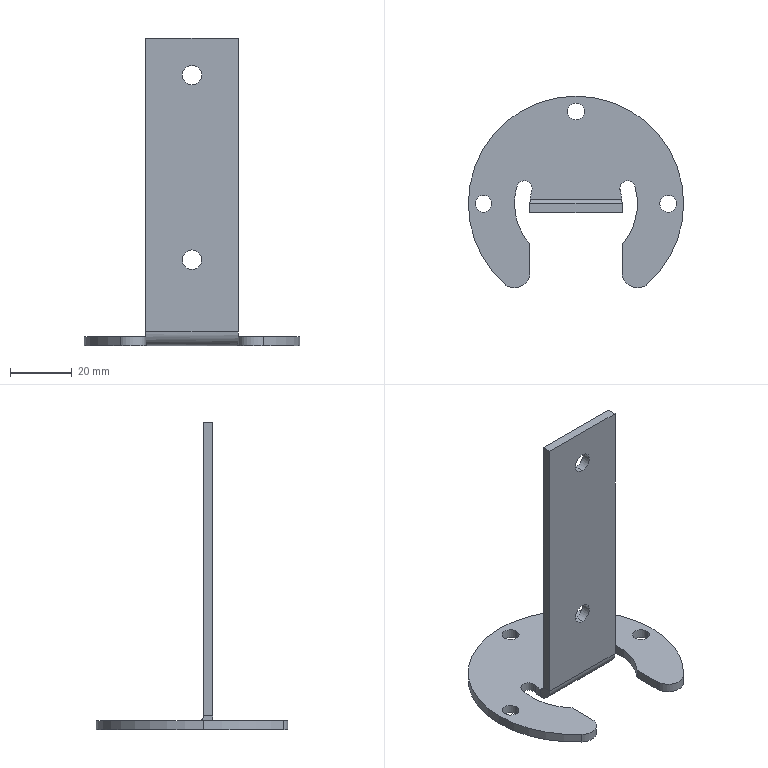Part | STEP file | Water guard support tab SGN-7-01 | 1 solid | 36 faces | box 70 x 62.361 x 100 mm | volume 16365 mm3 | cylinder 25 | plane 9 | spline 2 | commonest cylinder face diameters 5.5 x6 6.3 x4 5 x3 40 x3 70 x3 10 x2